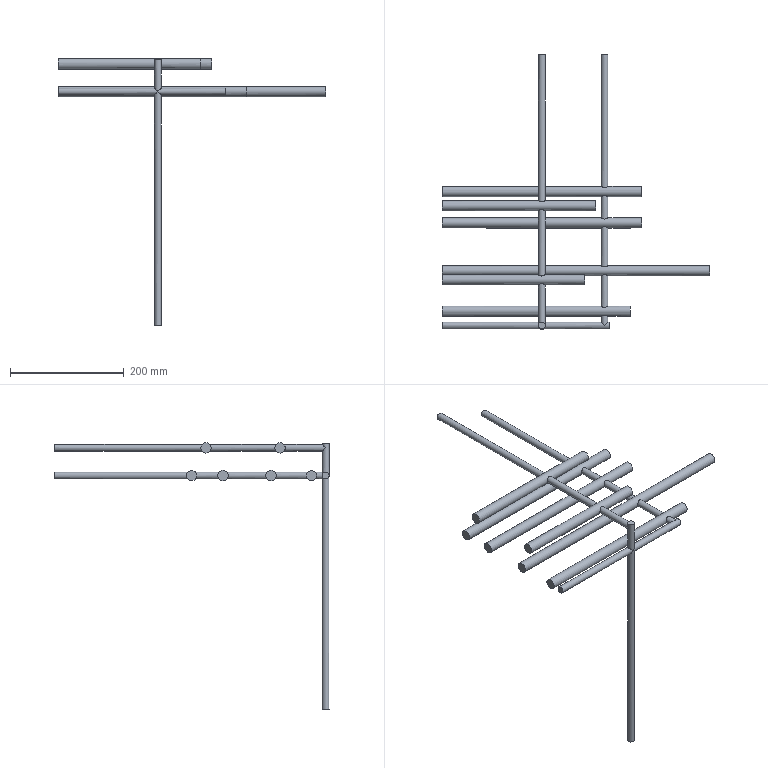Part | STEP file | solid 212 | 1 solid | 36 faces | box 470 x 481 x 467.5 mm | volume 693577 mm3 | cylinder 18 | plane 18 | commonest cylinder face diameters 12 x12 18 x6